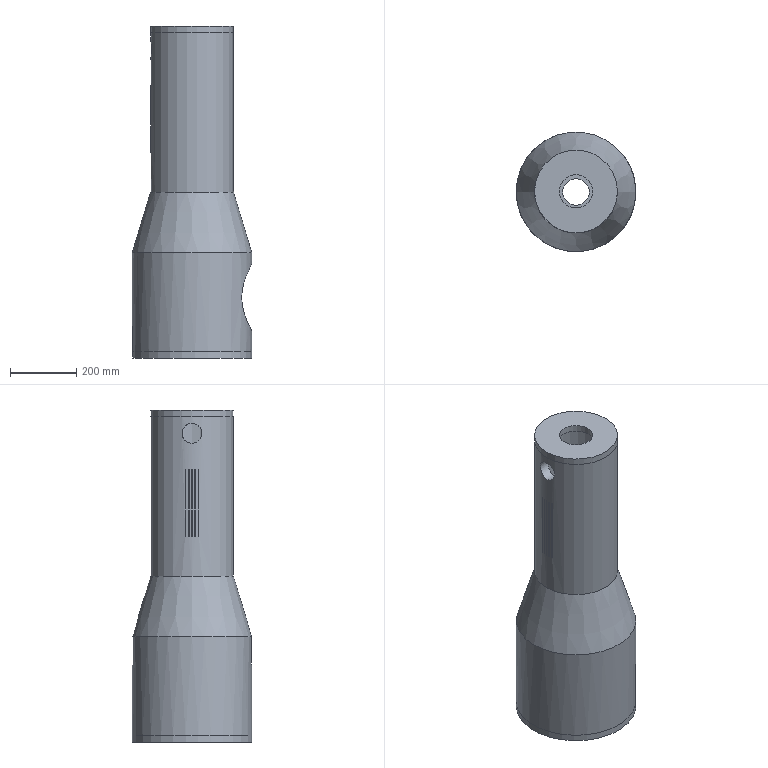Part | NX | features CYLINDER 4, DATUM_CSYS 4, EXTRUDE 3, SKETCH 3, SPLIT BODY 2, CHAMFER 1, SHELL 1 | 3 solids | 38 faces | box 360 x 360 x 1000 mm | volume 21575281 mm3 | plane 26 | cylinder 10 | cone 2 | commonest cylinder face diameters 250 x2 360 x2 60 x1 80 x1 100 x1 190 x1
STEP:
#1=CARTESIAN_POINT('',(-95.,0.,600.));
#2=VERTEX_POINT('',#1);
#3=CARTESIAN_POINT('',(-94.478,11.872,601.599));
#4=CARTESIAN_POINT('',(-95.261,-0.00341,599.201));
#5=CARTESIAN_POINT('',(-94.479,-11.859,601.595));
#6=CARTESIAN_POINT('',(-92.607,-21.764,608.254));
#7=CARTESIAN_POINT('',(-90.692,-28.404,618.148));
#8=CARTESIAN_POINT('',(-89.863,-30.794,629.974));
#9=CARTESIAN_POINT('',(-90.688,-28.419,641.834));
#10=CARTESIAN_POINT('',(-92.61,-21.752,651.761));
#11=CARTESIAN_POINT('',(-94.48,-11.846,658.408));
#12=CARTESIAN_POINT('',(-95.259,-0.01477,660.794));
#13=CARTESIAN_POINT('',(-94.483,11.831,658.417));
#14=CARTESIAN_POINT('',(-92.611,21.751,651.762));
#15=CARTESIAN_POINT('',(-90.691,28.408,641.851));
#16=CARTESIAN_POINT('',(-89.863,30.795,630.006));
#17=CARTESIAN_POINT('',(-90.69,28.413,618.159));
#18=CARTESIAN_POINT('',(-92.607,21.762,608.254));
#19=CARTESIAN_POINT('',(-94.478,11.872,601.599));
#20=CARTESIAN_POINT('',(-95.261,-0.00341,599.201));
#21=CARTESIAN_POINT('',(-94.479,-11.859,601.595));
#22=B_SPLINE_CURVE_WITH_KNOTS('',3,(#3,#4,#5,#6,#7,#8,#9,#10,#11,#12,#13,#14,#15,#16,#17,#18,#19,#20,#21),.UNSPECIFIED.,.T.,.F.,(1,1,1,1,1,1,1,1,1,1,1,1,1,1,1,1,1,1,1,1,1,1,1),(-0.0354,-0.0236,-0.0118,0.,0.0118,0.0236,0.0354,0.04719,0.05899,0.07079,0.08259,0.09439,0.1062,0.118,0.1298,0.1416,0.1534,0.1652,0.177,0.1888,0.2006,0.2124,0.2242),.UNSPECIFIED.);
#23=EDGE_CURVE('',#2,#2,#22,.T.);
#24=ORIENTED_EDGE('',*,*,#23,.T.);
#25=EDGE_LOOP('',(#24));
#26=FACE_BOUND('',#25,.T.);
#27=CARTESIAN_POINT('',(-94.573,9.,520.));
#28=VERTEX_POINT('',#27);
#29=CARTESIAN_POINT('',(-94.573,9.,320.));
#30=VERTEX_POINT('',#29);
#31=CARTESIAN_POINT('',(-94.573,9.,0.));
#32=DIRECTION('',(0.,0.,1.));
#33=VECTOR('',#32,1000.);
#34=LINE('',#31,#33);
#35=EDGE_CURVE('',#28,#30,#34,.F.);
#36=ORIENTED_EDGE('',*,*,#35,.F.);
#37=CARTESIAN_POINT('',(-94.361,11.,520.));
#38=VERTEX_POINT('',#37);
#39=CARTESIAN_POINT('',(0.,0.,520.));
#40=DIRECTION('',(0.,0.,1.));
#41=DIRECTION('',(1.,0.,0.));
#42=AXIS2_PLACEMENT_3D('',#39,#40,#41);
#43=CIRCLE('',#42,95.);
#44=EDGE_CURVE('',#38,#28,#43,.T.);
#45=ORIENTED_EDGE('',*,*,#44,.F.);
#46=CARTESIAN_POINT('',(-94.361,11.,320.));
#47=VERTEX_POINT('',#46);
#48=CARTESIAN_POINT('',(-94.361,11.,0.));
#49=DIRECTION('',(0.,0.,1.));
#50=VECTOR('',#49,1000.);
#51=LINE('',#48,#50);
#52=EDGE_CURVE('',#47,#38,#51,.T.);
#53=ORIENTED_EDGE('',*,*,#52,.F.);
#54=CARTESIAN_POINT('',(0.,0.,320.));
#55=DIRECTION('',(0.,0.,-1.));
#56=DIRECTION('',(-1.,0.,0.));
#57=AXIS2_PLACEMENT_3D('',#54,#55,#56);
#58=CIRCLE('',#57,95.);
#59=EDGE_CURVE('',#30,#47,#58,.T.);
#60=ORIENTED_EDGE('',*,*,#59,.F.);
#61=EDGE_LOOP('',(#36,#45,#53,#60));
#62=FACE_BOUND('',#61,.T.);
#63=CARTESIAN_POINT('',(-92.65,-21.,520.));
#64=VERTEX_POINT('',#63);
#65=CARTESIAN_POINT('',(-92.65,-21.,320.));
#66=VERTEX_POINT('',#65);
#67=CARTESIAN_POINT('',(-92.65,-21.,0.));
#68=DIRECTION('',(0.,0.,1.));
#69=VECTOR('',#68,1000.);
#70=LINE('',#67,#69);
#71=EDGE_CURVE('',#64,#66,#70,.F.);
#72=ORIENTED_EDGE('',*,*,#71,.F.);
#73=CARTESIAN_POINT('',(-93.081,-19.,520.));
#74=VERTEX_POINT('',#73);
#75=CARTESIAN_POINT('',(0.,0.,520.));
#76=DIRECTION('',(0.,0.,1.));
#77=DIRECTION('',(1.,0.,0.));
#78=AXIS2_PLACEMENT_3D('',#75,#76,#77);
#79=CIRCLE('',#78,95.);
#80=EDGE_CURVE('',#74,#64,#79,.T.);
#81=ORIENTED_EDGE('',*,*,#80,.F.);
#82=CARTESIAN_POINT('',(-93.081,-19.,320.));
#83=VERTEX_POINT('',#82);
#84=CARTESIAN_POINT('',(-93.081,-19.,0.));
#85=DIRECTION('',(0.,0.,1.));
#86=VECTOR('',#85,1000.);
#87=LINE('',#84,#86);
#88=EDGE_CURVE('',#83,#74,#87,.T.);
#89=ORIENTED_EDGE('',*,*,#88,.F.);
#90=CARTESIAN_POINT('',(0.,0.,320.));
#91=DIRECTION('',(0.,0.,-1.));
#92=DIRECTION('',(-1.,0.,0.));
#93=AXIS2_PLACEMENT_3D('',#90,#91,#92);
#94=CIRCLE('',#93,95.);
#95=EDGE_CURVE('',#66,#83,#94,.T.);
#96=ORIENTED_EDGE('',*,*,#95,.F.);
#97=EDGE_LOOP('',(#72,#81,#89,#96));
#98=FACE_BOUND('',#97,.T.);
#99=CARTESIAN_POINT('',(-94.995,1.,320.));
#100=VERTEX_POINT('',#99);
#101=CARTESIAN_POINT('',(-94.995,-1.,320.));
#102=VERTEX_POINT('',#101);
#103=CARTESIAN_POINT('',(0.,0.,320.));
#104=DIRECTION('',(0.,0.,-1.));
#105=DIRECTION('',(-1.,0.,0.));
#106=AXIS2_PLACEMENT_3D('',#103,#104,#105);
#107=CIRCLE('',#106,95.);
#108=EDGE_CURVE('',#100,#102,#107,.F.);
#109=ORIENTED_EDGE('',*,*,#108,.T.);
#110=CARTESIAN_POINT('',(-94.995,-1.,520.));
#111=VERTEX_POINT('',#110);
#112=CARTESIAN_POINT('',(-94.995,-1.,0.));
#113=DIRECTION('',(0.,0.,1.));
#114=VECTOR('',#113,1000.);
#115=LINE('',#112,#114);
#116=EDGE_CURVE('',#102,#111,#115,.T.);
#117=ORIENTED_EDGE('',*,*,#116,.T.);
#118=CARTESIAN_POINT('',(-94.995,1.,520.));
#119=VERTEX_POINT('',#118);
#120=CARTESIAN_POINT('',(0.,0.,520.));
#121=DIRECTION('',(0.,0.,1.));
#122=DIRECTION('',(1.,0.,0.));
#123=AXIS2_PLACEMENT_3D('',#120,#121,#122);
#124=CIRCLE('',#123,95.);
#125=EDGE_CURVE('',#111,#119,#124,.F.);
#126=ORIENTED_EDGE('',*,*,#125,.T.);
#127=CARTESIAN_POINT('',(-94.995,1.,0.));
#128=DIRECTION('',(0.,0.,1.));
#129=VECTOR('',#128,1000.);
#130=LINE('',#127,#129);
#131=EDGE_CURVE('',#119,#100,#130,.F.);
#132=ORIENTED_EDGE('',*,*,#131,.T.);
#133=EDGE_LOOP('',(#109,#117,#126,#132));
#134=FACE_BOUND('',#133,.T.);
#135=CARTESIAN_POINT('',(-95.,0.,230.398));
#136=VERTEX_POINT('',#135);
#137=CARTESIAN_POINT('',(0.,0.,230.398));
#138=DIRECTION('',(0.,0.,-1.));
#139=DIRECTION('',(-1.,0.,0.));
#140=AXIS2_PLACEMENT_3D('',#137,#138,#139);
#141=CIRCLE('',#140,95.);
#142=EDGE_CURVE('',#136,#136,#141,.F.);
#143=ORIENTED_EDGE('',*,*,#142,.F.);
#144=EDGE_LOOP('',(#143));
#145=FACE_BOUND('',#144,.T.);
#146=CARTESIAN_POINT('',(95.,0.,680.));
#147=VERTEX_POINT('',#146);
#148=CARTESIAN_POINT('',(0.,0.,680.));
#149=DIRECTION('',(0.,0.,1.));
#150=DIRECTION('',(1.,0.,0.));
#151=AXIS2_PLACEMENT_3D('',#148,#149,#150);
#152=CIRCLE('',#151,95.);
#153=EDGE_CURVE('',#147,#147,#152,.F.);
#154=ORIENTED_EDGE('',*,*,#153,.F.);
#155=EDGE_LOOP('',(#154));
#156=FACE_BOUND('',#155,.T.);
#157=CARTESIAN_POINT('',(-94.361,-11.,520.));
#158=VERTEX_POINT('',#157);
#159=CARTESIAN_POINT('',(-94.361,-11.,320.));
#160=VERTEX_POINT('',#159);
#161=CARTESIAN_POINT('',(-94.361,-11.,0.));
#162=DIRECTION('',(0.,0.,1.));
#163=VECTOR('',#162,1000.);
#164=LINE('',#161,#163);
#165=EDGE_CURVE('',#158,#160,#164,.F.);
#166=ORIENTED_EDGE('',*,*,#165,.F.);
#167=CARTESIAN_POINT('',(-94.573,-9.,520.));
#168=VERTEX_POINT('',#167);
#169=CARTESIAN_POINT('',(0.,0.,520.));
#170=DIRECTION('',(0.,0.,1.));
#171=DIRECTION('',(1.,0.,0.));
#172=AXIS2_PLACEMENT_3D('',#169,#170,#171);
#173=CIRCLE('',#172,95.);
#174=EDGE_CURVE('',#168,#158,#173,.T.);
#175=ORIENTED_EDGE('',*,*,#174,.F.);
#176=CARTESIAN_POINT('',(-94.573,-9.,320.));
#177=VERTEX_POINT('',#176);
#178=CARTESIAN_POINT('',(-94.573,-9.,0.));
#179=DIRECTION('',(0.,0.,1.));
#180=VECTOR('',#179,1000.);
#181=LINE('',#178,#180);
#182=EDGE_CURVE('',#177,#168,#181,.T.);
#183=ORIENTED_EDGE('',*,*,#182,.F.);
#184=CARTESIAN_POINT('',(0.,0.,320.));
#185=DIRECTION('',(0.,0.,-1.));
#186=DIRECTION('',(-1.,0.,0.));
#187=AXIS2_PLACEMENT_3D('',#184,#185,#186);
#188=CIRCLE('',#187,95.);
#189=EDGE_CURVE('',#160,#177,#188,.T.);
#190=ORIENTED_EDGE('',*,*,#189,.F.);
#191=EDGE_LOOP('',(#166,#175,#183,#190));
#192=FACE_BOUND('',#191,.T.);
#193=CARTESIAN_POINT('',(-93.081,19.,520.));
#194=VERTEX_POINT('',#193);
#195=CARTESIAN_POINT('',(-93.081,19.,320.));
#196=VERTEX_POINT('',#195);
#197=CARTESIAN_POINT('',(-93.081,19.,0.));
#198=DIRECTION('',(0.,0.,1.));
#199=VECTOR('',#198,1000.);
#200=LINE('',#197,#199);
#201=EDGE_CURVE('',#194,#196,#200,.F.);
#202=ORIENTED_EDGE('',*,*,#201,.F.);
#203=CARTESIAN_POINT('',(-92.65,21.,520.));
#204=VERTEX_POINT('',#203);
#205=CARTESIAN_POINT('',(0.,0.,520.));
#206=DIRECTION('',(0.,0.,1.));
#207=DIRECTION('',(1.,0.,0.));
#208=AXIS2_PLACEMENT_3D('',#205,#206,#207);
#209=CIRCLE('',#208,95.);
#210=EDGE_CURVE('',#204,#194,#209,.T.);
#211=ORIENTED_EDGE('',*,*,#210,.F.);
#212=CARTESIAN_POINT('',(-92.65,21.,320.));
#213=VERTEX_POINT('',#212);
#214=CARTESIAN_POINT('',(-92.65,21.,0.));
#215=DIRECTION('',(0.,0.,1.));
#216=VECTOR('',#215,1000.);
#217=LINE('',#214,#216);
#218=EDGE_CURVE('',#213,#204,#217,.T.);
#219=ORIENTED_EDGE('',*,*,#218,.F.);
#220=CARTESIAN_POINT('',(0.,0.,320.));
#221=DIRECTION('',(0.,0.,-1.));
#222=DIRECTION('',(-1.,0.,0.));
#223=AXIS2_PLACEMENT_3D('',#220,#221,#222);
#224=CIRCLE('',#223,95.);
#225=EDGE_CURVE('',#196,#213,#224,.T.);
#226=ORIENTED_EDGE('',*,*,#225,.F.);
#227=EDGE_LOOP('',(#202,#211,#219,#226));
#228=FACE_BOUND('',#227,.T.);
#229=CARTESIAN_POINT('',(0.,0.,0.));
#230=DIRECTION('',(0.,0.,1.));
#231=DIRECTION('',(1.,0.,0.));
#232=AXIS2_PLACEMENT_3D('',#229,#230,#231);
#233=CYLINDRICAL_SURFACE('',#232,95.);
#234=ADVANCED_FACE('',(#26,#62,#98,#134,#145,#156,#192,#228),#233,.F.);
#235=CARTESIAN_POINT('',(-125.,0.,600.));
#236=VERTEX_POINT('',#235);
#237=CARTESIAN_POINT('',(-124.604,11.861,601.594));
#238=CARTESIAN_POINT('',(-125.197,-0.008703,599.206));
#239=CARTESIAN_POINT('',(-124.606,-11.826,601.583));
#240=CARTESIAN_POINT('',(-123.189,-21.765,608.246));
#241=CARTESIAN_POINT('',(-121.754,-28.417,618.177));
#242=CARTESIAN_POINT('',(-121.144,-30.788,629.978));
#243=CARTESIAN_POINT('',(-121.75,-28.432,641.799));
#244=CARTESIAN_POINT('',(-123.19,-21.761,651.761));
#245=CARTESIAN_POINT('',(-124.607,-11.819,658.42));
#246=CARTESIAN_POINT('',(-125.196,-0.01358,660.788));
#247=CARTESIAN_POINT('',(-124.609,11.798,658.43));
#248=CARTESIAN_POINT('',(-123.193,21.743,651.776));
#249=CARTESIAN_POINT('',(-121.755,28.412,641.843));
#250=CARTESIAN_POINT('',(-121.143,30.79,630.016));
#251=CARTESIAN_POINT('',(-121.752,28.428,618.195));
#252=CARTESIAN_POINT('',(-123.188,21.77,608.255));
#253=CARTESIAN_POINT('',(-124.604,11.861,601.594));
#254=CARTESIAN_POINT('',(-125.197,-0.008703,599.206));
#255=CARTESIAN_POINT('',(-124.606,-11.826,601.583));
#256=B_SPLINE_CURVE_WITH_KNOTS('',3,(#237,#238,#239,#240,#241,#242,#243,#244,#245,#246,#247,#248,#249,#250,#251,#252,#253,#254,#255),.UNSPECIFIED.,.T.,.F.,(1,1,1,1,1,1,1,1,1,1,1,1,1,1,1,1,1,1,1,1,1,1,1),(-0.0353,-0.02353,-0.01177,0.,0.01177,0.02353,0.0353,0.04706,0.05883,0.07059,0.08236,0.09413,0.1059,0.1177,0.1294,0.1412,0.153,0.1647,0.1765,0.1883,0.2,0.2118,0.2235),.UNSPECIFIED.);
#257=EDGE_CURVE('',#236,#236,#256,.T.);
#258=ORIENTED_EDGE('',*,*,#257,.F.);
#259=EDGE_LOOP('',(#258));
#260=FACE_BOUND('',#259,.T.);
#261=CARTESIAN_POINT('',(-124.996,-1.,320.));
#262=VERTEX_POINT('',#261);
#263=CARTESIAN_POINT('',(-124.996,-1.,520.));
#264=VERTEX_POINT('',#263);
#265=CARTESIAN_POINT('',(-124.996,-1.,0.));
#266=DIRECTION('',(0.,0.,1.));
#267=VECTOR('',#266,1000.);
#268=LINE('',#265,#267);
#269=EDGE_CURVE('',#262,#264,#268,.T.);
#270=ORIENTED_EDGE('',*,*,#269,.F.);
#271=CARTESIAN_POINT('',(-124.996,1.,320.));
#272=VERTEX_POINT('',#271);
#273=CARTESIAN_POINT('',(0.,0.,320.));
#274=DIRECTION('',(0.,0.,-1.));
#275=DIRECTION('',(-1.,0.,0.));
#276=AXIS2_PLACEMENT_3D('',#273,#274,#275);
#277=CIRCLE('',#276,125.);
#278=EDGE_CURVE('',#272,#262,#277,.F.);
#279=ORIENTED_EDGE('',*,*,#278,.F.);
#280=CARTESIAN_POINT('',(-124.996,1.,520.));
#281=VERTEX_POINT('',#280);
#282=CARTESIAN_POINT('',(-124.996,1.,0.));
#283=DIRECTION('',(0.,0.,1.));
#284=VECTOR('',#283,1000.);
#285=LINE('',#282,#284);
#286=EDGE_CURVE('',#281,#272,#285,.F.);
#287=ORIENTED_EDGE('',*,*,#286,.F.);
#288=CARTESIAN_POINT('',(0.,0.,520.));
#289=DIRECTION('',(0.,0.,1.));
#290=DIRECTION('',(1.,0.,0.));
#291=AXIS2_PLACEMENT_3D('',#288,#289,#290);
#292=CIRCLE('',#291,125.);
#293=EDGE_CURVE('',#264,#281,#292,.F.);
#294=ORIENTED_EDGE('',*,*,#293,.F.);
#295=EDGE_LOOP('',(#270,#279,#287,#294));
#296=FACE_BOUND('',#295,.T.);
#297=CARTESIAN_POINT('',(-125.,0.,680.));
#298=VERTEX_POINT('',#297);
#299=CARTESIAN_POINT('',(0.,0.,680.));
#300=DIRECTION('',(0.,0.,-1.));
#301=DIRECTION('',(-1.,0.,0.));
#302=AXIS2_PLACEMENT_3D('',#299,#300,#301);
#303=CIRCLE('',#302,125.);
#304=EDGE_CURVE('',#298,#298,#303,.F.);
#305=ORIENTED_EDGE('',*,*,#304,.F.);
#306=EDGE_LOOP('',(#305));
#307=FACE_BOUND('',#306,.T.);
#308=CARTESIAN_POINT('',(125.,0.,200.));
#309=VERTEX_POINT('',#308);
#310=CARTESIAN_POINT('',(0.,0.,200.));
#311=DIRECTION('',(0.,0.,1.));
#312=DIRECTION('',(1.,0.,0.));
#313=AXIS2_PLACEMENT_3D('',#310,#311,#312);
#314=CIRCLE('',#313,125.);
#315=EDGE_CURVE('',#309,#309,#314,.T.);
#316=ORIENTED_EDGE('',*,*,#315,.T.);
#317=EDGE_LOOP('',(#316));
#318=FACE_BOUND('',#317,.T.);
#319=CARTESIAN_POINT('',(-123.548,-19.,520.));
#320=VERTEX_POINT('',#319);
#321=CARTESIAN_POINT('',(-123.223,-21.,520.));
#322=VERTEX_POINT('',#321);
#323=CARTESIAN_POINT('',(0.,0.,520.));
#324=DIRECTION('',(0.,0.,1.));
#325=DIRECTION('',(1.,0.,0.));
#326=AXIS2_PLACEMENT_3D('',#323,#324,#325);
#327=CIRCLE('',#326,125.);
#328=EDGE_CURVE('',#320,#322,#327,.T.);
#329=ORIENTED_EDGE('',*,*,#328,.T.);
#330=CARTESIAN_POINT('',(-123.223,-21.,320.));
#331=VERTEX_POINT('',#330);
#332=CARTESIAN_POINT('',(-123.223,-21.,0.));
#333=DIRECTION('',(0.,0.,1.));
#334=VECTOR('',#333,1000.);
#335=LINE('',#332,#334);
#336=EDGE_CURVE('',#322,#331,#335,.F.);
#337=ORIENTED_EDGE('',*,*,#336,.T.);
#338=CARTESIAN_POINT('',(-123.548,-19.,320.));
#339=VERTEX_POINT('',#338);
#340=CARTESIAN_POINT('',(0.,0.,320.));
#341=DIRECTION('',(0.,0.,-1.));
#342=DIRECTION('',(-1.,0.,0.));
#343=AXIS2_PLACEMENT_3D('',#340,#341,#342);
#344=CIRCLE('',#343,125.);
#345=EDGE_CURVE('',#331,#339,#344,.T.);
#346=ORIENTED_EDGE('',*,*,#345,.T.);
#347=CARTESIAN_POINT('',(-123.548,-19.,0.));
#348=DIRECTION('',(0.,0.,1.));
#349=VECTOR('',#348,1000.);
#350=LINE('',#347,#349);
#351=EDGE_CURVE('',#339,#320,#350,.T.);
#352=ORIENTED_EDGE('',*,*,#351,.T.);
#353=EDGE_LOOP('',(#329,#337,#346,#352));
#354=FACE_BOUND('',#353,.T.);
#355=CARTESIAN_POINT('',(-124.676,-9.,520.));
#356=VERTEX_POINT('',#355);
#357=CARTESIAN_POINT('',(-124.515,-11.,520.));
#358=VERTEX_POINT('',#357);
#359=CARTESIAN_POINT('',(0.,0.,520.));
#360=DIRECTION('',(0.,0.,1.));
#361=DIRECTION('',(1.,0.,0.));
#362=AXIS2_PLACEMENT_3D('',#359,#360,#361);
#363=CIRCLE('',#362,125.);
#364=EDGE_CURVE('',#356,#358,#363,.T.);
#365=ORIENTED_EDGE('',*,*,#364,.T.);
#366=CARTESIAN_POINT('',(-124.515,-11.,320.));
#367=VERTEX_POINT('',#366);
#368=CARTESIAN_POINT('',(-124.515,-11.,0.));
#369=DIRECTION('',(0.,0.,1.));
#370=VECTOR('',#369,1000.);
#371=LINE('',#368,#370);
#372=EDGE_CURVE('',#358,#367,#371,.F.);
#373=ORIENTED_EDGE('',*,*,#372,.T.);
#374=CARTESIAN_POINT('',(-124.676,-9.,320.));
#375=VERTEX_POINT('',#374);
#376=CARTESIAN_POINT('',(0.,0.,320.));
#377=DIRECTION('',(0.,0.,-1.));
#378=DIRECTION('',(-1.,0.,0.));
#379=AXIS2_PLACEMENT_3D('',#376,#377,#378);
#380=CIRCLE('',#379,125.);
#381=EDGE_CURVE('',#367,#375,#380,.T.);
#382=ORIENTED_EDGE('',*,*,#381,.T.);
#383=CARTESIAN_POINT('',(-124.676,-9.,0.));
#384=DIRECTION('',(0.,0.,1.));
#385=VECTOR('',#384,1000.);
#386=LINE('',#383,#385);
#387=EDGE_CURVE('',#375,#356,#386,.T.);
#388=ORIENTED_EDGE('',*,*,#387,.T.);
#389=EDGE_LOOP('',(#365,#373,#382,#388));
#390=FACE_BOUND('',#389,.T.);
#391=CARTESIAN_POINT('',(-124.515,11.,520.));
#392=VERTEX_POINT('',#391);
#393=CARTESIAN_POINT('',(-124.676,9.,520.));
#394=VERTEX_POINT('',#393);
#395=CARTESIAN_POINT('',(0.,0.,520.));
#396=DIRECTION('',(0.,0.,1.));
#397=DIRECTION('',(1.,0.,0.));
#398=AXIS2_PLACEMENT_3D('',#395,#396,#397);
#399=CIRCLE('',#398,125.);
#400=EDGE_CURVE('',#392,#394,#399,.T.);
#401=ORIENTED_EDGE('',*,*,#400,.T.);
#402=CARTESIAN_POINT('',(-124.676,9.,320.));
#403=VERTEX_POINT('',#402);
#404=CARTESIAN_POINT('',(-124.676,9.,0.));
#405=DIRECTION('',(0.,0.,1.));
#406=VECTOR('',#405,1000.);
#407=LINE('',#404,#406);
#408=EDGE_CURVE('',#394,#403,#407,.F.);
#409=ORIENTED_EDGE('',*,*,#408,.T.);
#410=CARTESIAN_POINT('',(-124.515,11.,320.));
#411=VERTEX_POINT('',#410);
#412=CARTESIAN_POINT('',(0.,0.,320.));
#413=DIRECTION('',(0.,0.,-1.));
#414=DIRECTION('',(-1.,0.,0.));
#415=AXIS2_PLACEMENT_3D('',#412,#413,#414);
#416=CIRCLE('',#415,125.);
#417=EDGE_CURVE('',#403,#411,#416,.T.);
#418=ORIENTED_EDGE('',*,*,#417,.T.);
#419=CARTESIAN_POINT('',(-124.515,11.,0.));
#420=DIRECTION('',(0.,0.,1.));
#421=VECTOR('',#420,1000.);
#422=LINE('',#419,#421);
#423=EDGE_CURVE('',#411,#392,#422,.T.);
#424=ORIENTED_EDGE('',*,*,#423,.T.);
#425=EDGE_LOOP('',(#401,#409,#418,#424));
#426=FACE_BOUND('',#425,.T.);
#427=CARTESIAN_POINT('',(-123.223,21.,520.));
#428=VERTEX_POINT('',#427);
#429=CARTESIAN_POINT('',(-123.548,19.,520.));
#430=VERTEX_POINT('',#429);
#431=CARTESIAN_POINT('',(0.,0.,520.));
#432=DIRECTION('',(0.,0.,1.));
#433=DIRECTION('',(1.,0.,0.));
#434=AXIS2_PLACEMENT_3D('',#431,#432,#433);
#435=CIRCLE('',#434,125.);
#436=EDGE_CURVE('',#428,#430,#435,.T.);
#437=ORIENTED_EDGE('',*,*,#436,.T.);
#438=CARTESIAN_POINT('',(-123.548,19.,320.));
#439=VERTEX_POINT('',#438);
#440=CARTESIAN_POINT('',(-123.548,19.,0.));
#441=DIRECTION('',(0.,0.,1.));
#442=VECTOR('',#441,1000.);
#443=LINE('',#440,#442);
#444=EDGE_CURVE('',#430,#439,#443,.F.);
#445=ORIENTED_EDGE('',*,*,#444,.T.);
#446=CARTESIAN_POINT('',(-123.223,21.,320.));
#447=VERTEX_POINT('',#446);
#448=CARTESIAN_POINT('',(0.,0.,320.));
#449=DIRECTION('',(0.,0.,-1.));
#450=DIRECTION('',(-1.,0.,0.));
#451=AXIS2_PLACEMENT_3D('',#448,#449,#450);
#452=CIRCLE('',#451,125.);
#453=EDGE_CURVE('',#439,#447,#452,.T.);
#454=ORIENTED_EDGE('',*,*,#453,.T.);
#455=CARTESIAN_POINT('',(-123.223,21.,0.));
#456=DIRECTION('',(0.,0.,1.));
#457=VECTOR('',#456,1000.);
#458=LINE('',#455,#457);
#459=EDGE_CURVE('',#447,#428,#458,.T.);
#460=ORIENTED_EDGE('',*,*,#459,.T.);
#461=EDGE_LOOP('',(#437,#445,#454,#460));
#462=FACE_BOUND('',#461,.T.);
#463=CARTESIAN_POINT('',(0.,0.,0.));
#464=DIRECTION('',(0.,0.,1.));
#465=DIRECTION('',(1.,0.,0.));
#466=AXIS2_PLACEMENT_3D('',#463,#464,#465);
#467=CYLINDRICAL_SURFACE('',#466,125.);
#468=ADVANCED_FACE('',(#260,#296,#307,#318,#354,#390,#426,#462),#467,.T.);
#469=CARTESIAN_POINT('',(160.,0.,-17.617));
#470=VERTEX_POINT('',#469);
#471=CARTESIAN_POINT('',(159.099,20.518,-19.051));
#472=CARTESIAN_POINT('',(160.439,-0.1034,-16.918));
#473=CARTESIAN_POINT('',(159.145,-20.104,-18.977));
#474=CARTESIAN_POINT('',(156.082,-36.139,-23.971));
#475=CARTESIAN_POINT('',(152.77,-47.832,-29.62));
#476=CARTESIAN_POINT('',(149.907,-56.148,-34.677));
#477=CARTESIAN_POINT('',(146.77,-63.875,-40.477));
#478=CARTESIAN_POINT('',(143.498,-70.901,-46.885));
#479=CARTESIAN_POINT('',(140.142,-77.308,-53.943));
#480=CARTESIAN_POINT('',(135.688,-84.973,-64.228));
#481=CARTESIAN_POINT('',(130.613,-92.568,-78.149));
#482=CARTESIAN_POINT('',(126.812,-97.586,-94.068));
#483=CARTESIAN_POINT('',(125.2,-99.627,-107.205));
#484=CARTESIAN_POINT('',(124.615,-100.352,-120.826));
#485=CARTESIAN_POINT('',(125.697,-99.022,-134.142));
#486=CARTESIAN_POINT('',(128.229,-95.717,-147.132));
#487=CARTESIAN_POINT('',(131.48,-91.262,-159.395));
#488=CARTESIAN_POINT('',(136.655,-83.532,-173.697));
#489=CARTESIAN_POINT('',(142.28,-73.495,-185.953));
#490=CARTESIAN_POINT('',(146.709,-64.017,-194.64));
#491=CARTESIAN_POINT('',(149.814,-56.386,-200.387));
#492=CARTESIAN_POINT('',(152.658,-48.191,-205.419));
#493=CARTESIAN_POINT('',(155.183,-39.341,-209.731));
#494=CARTESIAN_POINT('',(157.258,-30.015,-213.178));
#495=CARTESIAN_POINT('',(158.789,-20.444,-215.671));
#496=CARTESIAN_POINT('',(159.758,-10.572,-217.23));
#497=CARTESIAN_POINT('',(160.223,3.07,-217.972));
#498=CARTESIAN_POINT('',(159.402,16.372,-216.668));
#499=CARTESIAN_POINT('',(157.365,29.465,-213.353));
#500=CARTESIAN_POINT('',(155.328,38.755,-209.975));
#501=CARTESIAN_POINT('',(152.843,47.606,-205.742));
#502=CARTESIAN_POINT('',(149.005,58.786,-198.965));
#503=CARTESIAN_POINT('',(144.7,68.597,-190.869));
#504=CARTESIAN_POINT('',(140.176,77.247,-181.364));
#505=CARTESIAN_POINT('',(136.866,82.95,-173.736));
#506=CARTESIAN_POINT('',(133.716,87.921,-165.582));
#507=CARTESIAN_POINT('',(130.816,92.166,-156.831));
#508=CARTESIAN_POINT('',(128.328,95.585,-147.546));
#509=CARTESIAN_POINT('',(125.788,98.908,-134.799));
#510=CARTESIAN_POINT('',(124.63,100.334,-121.166));
#511=CARTESIAN_POINT('',(125.151,99.689,-107.816));
#512=CARTESIAN_POINT('',(126.74,97.678,-94.412));
#513=CARTESIAN_POINT('',(129.709,93.774,-81.822));
#514=CARTESIAN_POINT('',(133.58,88.129,-70.026));
#515=CARTESIAN_POINT('',(136.738,83.16,-61.808));
#516=CARTESIAN_POINT('',(140.058,77.46,-54.127));
#517=CARTESIAN_POINT('',(144.585,68.836,-44.591));
#518=CARTESIAN_POINT('',(149.963,56.656,-34.456));
#519=CARTESIAN_POINT('',(155.476,39.283,-24.958));
#520=CARTESIAN_POINT('',(159.099,20.518,-19.051));
#521=CARTESIAN_POINT('',(160.439,-0.1034,-16.918));
#522=CARTESIAN_POINT('',(159.145,-20.104,-18.977));
#523=B_SPLINE_CURVE_WITH_KNOTS('',3,(#471,#472,#473,#474,#475,#476,#477,#478,#479,#480,#481,#482,#483,#484,#485,#486,#487,#488,#489,#490,#491,#492,#493,#494,#495,#496,#497,#498,#499,#500,#501,#502,#503,#504,#505,#506,#507,#508,#509,#510,#511,#512,#513,#514,#515,#516,#517,#518,#519,#520,#521,#522),.UNSPECIFIED.,.T.,.F.,(1,1,1,1,1,1,1,1,1,1,1,1,1,1,1,1,1,1,1,1,1,1,1,1,1,1,1,1,1,1,1,1,1,1,1,1,1,1,1,1,1,1,1,1,1,1,1,1,1,1,1,1,1,1,1,1),(-0.06025,-0.04016,-0.02008,0.,0.02008,0.04016,0.05021,0.06025,0.07029,0.08033,0.09037,0.1004,0.1205,0.1406,0.1506,0.1607,0.1807,0.1908,0.2008,0.2209,0.241,0.251,0.2611,0.2711,0.2812,0.2912,0.3012,0.3113,0.3213,0.3414,0.3514,0.3615,0.3715,0.3816,0.4016,0.4117,0.4217,0.4318,0.4418,0.4518,0.4619,0.482,0.492,0.5021,0.5221,0.5322,0.5422,0.5523,0.5623,0.5824,0.6025,0.6225,0.6426,0.6627,0.6828,0.6928),.UNSPECIFIED.);
#524=EDGE_CURVE('',#470,#470,#523,.T.);
#525=ORIENTED_EDGE('',*,*,#524,.T.);
#526=EDGE_LOOP('',(#525));
#527=FACE_BOUND('',#526,.T.);
#528=CARTESIAN_POINT('',(-160.,0.,13.731));
#529=VERTEX_POINT('',#528);
#530=CARTESIAN_POINT('',(0.,0.,13.731));
#531=DIRECTION('',(0.,0.,-1.));
#532=DIRECTION('',(-1.,0.,0.));
#533=AXIS2_PLACEMENT_3D('',#530,#531,#532);
#534=CIRCLE('',#533,160.);
#535=EDGE_CURVE('',#529,#529,#534,.T.);
#536=ORIENTED_EDGE('',*,*,#535,.F.);
#537=EDGE_LOOP('',(#536));
#538=FACE_BOUND('',#537,.T.);
#539=CARTESIAN_POINT('',(-160.,0.,-280.));
#540=VERTEX_POINT('',#539);
#541=CARTESIAN_POINT('',(0.,0.,-280.));
#542=DIRECTION('',(0.,0.,-1.));
#543=DIRECTION('',(-1.,0.,0.));
#544=AXIS2_PLACEMENT_3D('',#541,#542,#543);
#545=CIRCLE('',#544,160.);
#546=EDGE_CURVE('',#540,#540,#545,.F.);
#547=ORIENTED_EDGE('',*,*,#546,.F.);
#548=EDGE_LOOP('',(#547));
#549=FACE_BOUND('',#548,.T.);
#550=CARTESIAN_POINT('',(0.,0.,0.));
#551=DIRECTION('',(0.,0.,-1.));
#552=DIRECTION('',(1.,0.,0.));
#553=AXIS2_PLACEMENT_3D('',#550,#551,#552);
#554=CYLINDRICAL_SURFACE('',#553,160.);
#555=ADVANCED_FACE('',(#527,#538,#549),#554,.F.);
#556=ORIENTED_EDGE('',*,*,#142,.T.);
#557=EDGE_LOOP('',(#556));
#558=FACE_BOUND('',#557,.T.);
#559=ORIENTED_EDGE('',*,*,#535,.T.);
#560=EDGE_LOOP('',(#559));
#561=FACE_BOUND('',#560,.T.);
#562=CARTESIAN_POINT('',(0.,0.,-5.747));
#563=DIRECTION('',(0.,0.,-1.));
#564=DIRECTION('',(-1.,0.,0.));
#565=AXIS2_PLACEMENT_3D('',#562,#563,#564);
#566=CONICAL_SURFACE('',#565,165.843,0.2915);
#567=ADVANCED_FACE('',(#558,#561),#566,.F.);
#568=CARTESIAN_POINT('',(180.,0.,-17.617));
#569=VERTEX_POINT('',#568);
#570=CARTESIAN_POINT('',(179.809,10.097,-17.96));
#571=CARTESIAN_POINT('',(180.095,-0.006015,-17.445));
#572=CARTESIAN_POINT('',(179.809,-10.073,-17.959));
#573=CARTESIAN_POINT('',(178.716,-23.155,-19.938));
#574=CARTESIAN_POINT('',(176.022,-39.153,-24.896));
#575=CARTESIAN_POINT('',(172.059,-53.393,-32.632));
#576=CARTESIAN_POINT('',(168.379,-63.795,-40.406));
#577=CARTESIAN_POINT('',(165.516,-70.869,-46.851));
#578=CARTESIAN_POINT('',(162.6,-77.308,-53.941));
#579=CARTESIAN_POINT('',(158.737,-85.044,-64.323));
#580=CARTESIAN_POINT('',(155.267,-91.139,-75.581));
#581=CARTESIAN_POINT('',(152.497,-95.649,-87.879));
#582=CARTESIAN_POINT('',(150.899,-98.139,-97.574));
#583=CARTESIAN_POINT('',(149.907,-99.641,-107.381));
#584=CARTESIAN_POINT('',(149.551,-100.171,-117.455));
#585=CARTESIAN_POINT('',(149.886,-99.673,-127.546));
#586=CARTESIAN_POINT('',(151.183,-97.71,-140.64));
#587=CARTESIAN_POINT('',(153.697,-93.771,-153.413));
#588=CARTESIAN_POINT('',(156.941,-88.198,-165.079));
#589=CARTESIAN_POINT('',(160.59,-81.476,-176.222));
#590=CARTESIAN_POINT('',(165.473,-71.362,-188.549));
#591=CARTESIAN_POINT('',(171.233,-56.34,-200.986));
#592=CARTESIAN_POINT('',(175.173,-42.221,-208.683));
#593=CARTESIAN_POINT('',(177.615,-29.737,-213.268));
#594=CARTESIAN_POINT('',(178.962,-20.108,-215.74));
#595=CARTESIAN_POINT('',(179.796,-10.31,-217.25));
#596=CARTESIAN_POINT('',(180.095,-0.2804,-217.787));
#597=CARTESIAN_POINT('',(179.823,9.851,-217.299));
#598=CARTESIAN_POINT('',(179.01,19.687,-215.827));
#599=CARTESIAN_POINT('',(177.677,29.363,-213.383));
#600=CARTESIAN_POINT('',(175.262,41.855,-208.853));
#601=CARTESIAN_POINT('',(172.094,53.283,-202.673));
#602=CARTESIAN_POINT('',(168.413,63.705,-194.902));
#603=CARTESIAN_POINT('',(165.548,70.795,-188.457));
#604=CARTESIAN_POINT('',(162.627,77.253,-181.361));
#605=CARTESIAN_POINT('',(158.757,85.006,-170.968));
#606=CARTESIAN_POINT('',(154.41,92.645,-156.918));
#607=CARTESIAN_POINT('',(151.233,97.634,-140.967));
#608=CARTESIAN_POINT('',(149.907,99.641,-127.862));
#609=CARTESIAN_POINT('',(149.551,100.172,-117.761));
#610=CARTESIAN_POINT('',(149.887,99.671,-107.671));
#611=CARTESIAN_POINT('',(151.188,97.702,-94.556));
#612=CARTESIAN_POINT('',(153.708,93.752,-81.77));
#613=CARTESIAN_POINT('',(156.961,88.164,-70.091));
#614=CARTESIAN_POINT('',(160.619,81.422,-58.933));
#615=CARTESIAN_POINT('',(165.507,71.286,-46.606));
#616=CARTESIAN_POINT('',(171.271,56.225,-34.168));
#617=CARTESIAN_POINT('',(175.209,42.075,-26.482));
#618=CARTESIAN_POINT('',(177.646,29.552,-21.908));
#619=CARTESIAN_POINT('',(178.984,19.914,-19.453));
#620=CARTESIAN_POINT('',(179.809,10.097,-17.96));
#621=CARTESIAN_POINT('',(180.095,-0.006015,-17.445));
#622=CARTESIAN_POINT('',(179.809,-10.073,-17.959));
#623=B_SPLINE_CURVE_WITH_KNOTS('',3,(#570,#571,#572,#573,#574,#575,#576,#577,#578,#579,#580,#581,#582,#583,#584,#585,#586,#587,#588,#589,#590,#591,#592,#593,#594,#595,#596,#597,#598,#599,#600,#601,#602,#603,#604,#605,#606,#607,#608,#609,#610,#611,#612,#613,#614,#615,#616,#617,#618,#619,#620,#621,#622),.UNSPECIFIED.,.T.,.F.,(1,1,1,1,1,1,1,1,1,1,1,1,1,1,1,1,1,1,1,1,1,1,1,1,1,1,1,1,1,1,1,1,1,1,1,1,1,1,1,1,1,1,1,1,1,1,1,1,1,1,1,1,1,1,1,1,1),(-0.02993,-0.01995,-0.009976,0.,0.009976,0.01995,0.0399,0.05986,0.06983,0.07981,0.08978,0.09976,0.1197,0.1297,0.1397,0.1496,0.1596,0.1696,0.1796,0.1995,0.2095,0.2195,0.2394,0.2594,0.2793,0.2893,0.2993,0.3093,0.3192,0.3292,0.3392,0.3492,0.3591,0.3791,0.3891,0.399,0.409,0.419,0.4389,0.4589,0.4689,0.4788,0.4888,0.4988,0.5187,0.5287,0.5387,0.5587,0.5786,0.5986,0.6085,0.6185,0.6285,0.6385,0.6484,0.6584,0.6784),.UNSPECIFIED.);
#624=EDGE_CURVE('',#569,#569,#623,.T.);
#625=ORIENTED_EDGE('',*,*,#624,.F.);
#626=EDGE_LOOP('',(#625));
#627=FACE_BOUND('',#626,.T.);
#628=CARTESIAN_POINT('',(180.,0.,-280.));
#629=VERTEX_POINT('',#628);
#630=CARTESIAN_POINT('',(0.,0.,-280.));
#631=DIRECTION('',(0.,0.,1.));
#632=DIRECTION('',(1.,0.,0.));
#633=AXIS2_PLACEMENT_3D('',#630,#631,#632);
#634=CIRCLE('',#633,180.);
#635=EDGE_CURVE('',#629,#629,#634,.F.);
#636=ORIENTED_EDGE('',*,*,#635,.F.);
#637=EDGE_LOOP('',(#636));
#638=FACE_BOUND('',#637,.T.);
#639=CARTESIAN_POINT('',(-180.,0.,16.667));
#640=VERTEX_POINT('',#639);
#641=CARTESIAN_POINT('',(0.,0.,16.667));
#642=DIRECTION('',(0.,0.,-1.));
#643=DIRECTION('',(-1.,0.,0.));
#644=AXIS2_PLACEMENT_3D('',#641,#642,#643);
#645=CIRCLE('',#644,180.);
#646=EDGE_CURVE('',#640,#640,#645,.T.);
#647=ORIENTED_EDGE('',*,*,#646,.T.);
#648=EDGE_LOOP('',(#647));
#649=FACE_BOUND('',#648,.T.);
#650=CARTESIAN_POINT('',(0.,0.,0.));
#651=DIRECTION('',(0.,0.,-1.));
#652=DIRECTION('',(1.,0.,0.));
#653=AXIS2_PLACEMENT_3D('',#650,#651,#652);
#654=CYLINDRICAL_SURFACE('',#653,180.);
#655=ADVANCED_FACE('',(#627,#638,#649),#654,.T.);
#656=ORIENTED_EDGE('',*,*,#315,.F.);
#657=EDGE_LOOP('',(#656));
#658=FACE_BOUND('',#657,.T.);
#659=ORIENTED_EDGE('',*,*,#646,.F.);
#660=EDGE_LOOP('',(#659));
#661=FACE_BOUND('',#660,.T.);
#662=CARTESIAN_POINT('',(0.,0.,0.));
#663=DIRECTION('',(0.,0.,-1.));
#664=DIRECTION('',(-1.,0.,0.));
#665=AXIS2_PLACEMENT_3D('',#662,#663,#664);
#666=CONICAL_SURFACE('',#665,185.,0.2915);
#667=ADVANCED_FACE('',(#658,#661),#666,.T.);
#668=ORIENTED_EDGE('',*,*,#546,.T.);
#669=EDGE_LOOP('',(#668));
#670=FACE_BOUND('',#669,.T.);
#671=ORIENTED_EDGE('',*,*,#635,.T.);
#672=EDGE_LOOP('',(#671));
#673=FACE_BOUND('',#672,.T.);
#674=CARTESIAN_POINT('',(0.,0.,-280.));
#675=DIRECTION('',(0.,0.,1.));
#676=DIRECTION('',(1.,0.,0.));
#677=AXIS2_PLACEMENT_3D('',#674,#675,#676);
#678=PLANE('',#677);
#679=ADVANCED_FACE('',(#670,#673),#678,.F.);
#680=ORIENTED_EDGE('',*,*,#153,.T.);
#681=EDGE_LOOP('',(#680));
#682=FACE_BOUND('',#681,.T.);
#683=ORIENTED_EDGE('',*,*,#304,.T.);
#684=EDGE_LOOP('',(#683));
#685=FACE_BOUND('',#684,.T.);
#686=CARTESIAN_POINT('',(0.,0.,680.));
#687=DIRECTION('',(0.,0.,-1.));
#688=DIRECTION('',(-1.,0.,0.));
#689=AXIS2_PLACEMENT_3D('',#686,#687,#688);
#690=PLANE('',#689);
#691=ADVANCED_FACE('',(#682,#685),#690,.F.);
#692=ORIENTED_EDGE('',*,*,#624,.T.);
#693=EDGE_LOOP('',(#692));
#694=FACE_BOUND('',#693,.T.);
#695=ORIENTED_EDGE('',*,*,#524,.F.);
#696=EDGE_LOOP('',(#695));
#697=FACE_BOUND('',#696,.T.);
#698=CARTESIAN_POINT('',(230.,0.,-117.617));
#699=DIRECTION('',(-1.,0.,0.));
#700=DIRECTION('',(0.,0.,1.));
#701=AXIS2_PLACEMENT_3D('',#698,#699,#700);
#702=CYLINDRICAL_SURFACE('',#701,100.);
#703=ADVANCED_FACE('',(#694,#697),#702,.F.);
#704=CARTESIAN_POINT('',(0.,-1.,320.));
#705=DIRECTION('',(1.,0.,0.));
#706=VECTOR('',#705,1000.);
#707=LINE('',#704,#706);
#708=EDGE_CURVE('',#102,#262,#707,.F.);
#709=ORIENTED_EDGE('',*,*,#708,.T.);
#710=ORIENTED_EDGE('',*,*,#269,.T.);
#711=CARTESIAN_POINT('',(0.,-1.,520.));
#712=DIRECTION('',(1.,0.,0.));
#713=VECTOR('',#712,1000.);
#714=LINE('',#711,#713);
#715=EDGE_CURVE('',#111,#264,#714,.F.);
#716=ORIENTED_EDGE('',*,*,#715,.F.);
#717=ORIENTED_EDGE('',*,*,#116,.F.);
#718=EDGE_LOOP('',(#709,#710,#716,#717));
#719=FACE_BOUND('',#718,.T.);
#720=CARTESIAN_POINT('',(0.,-1.,520.));
#721=DIRECTION('',(0.,-1.,0.));
#722=DIRECTION('',(0.,0.,-1.));
#723=AXIS2_PLACEMENT_3D('',#720,#721,#722);
#724=PLANE('',#723);
#725=ADVANCED_FACE('',(#719),#724,.F.);
#726=CARTESIAN_POINT('',(0.,1.,320.));
#727=DIRECTION('',(1.,0.,0.));
#728=VECTOR('',#727,1000.);
#729=LINE('',#726,#728);
#730=EDGE_CURVE('',#100,#272,#729,.F.);
#731=ORIENTED_EDGE('',*,*,#730,.T.);
#732=ORIENTED_EDGE('',*,*,#278,.T.);
#733=ORIENTED_EDGE('',*,*,#708,.F.);
#734=ORIENTED_EDGE('',*,*,#108,.F.);
#735=EDGE_LOOP('',(#731,#732,#733,#734));
#736=FACE_BOUND('',#735,.T.);
#737=CARTESIAN_POINT('',(0.,-1.,320.));
#738=DIRECTION('',(0.,0.,-1.));
#739=DIRECTION('',(-1.,0.,0.));
#740=AXIS2_PLACEMENT_3D('',#737,#738,#739);
#741=PLANE('',#740);
#742=ADVANCED_FACE('',(#736),#741,.F.);
#743=CARTESIAN_POINT('',(0.,1.,520.));
#744=DIRECTION('',(1.,0.,0.));
#745=VECTOR('',#744,1000.);
#746=LINE('',#743,#745);
#747=EDGE_CURVE('',#119,#281,#746,.F.);
#748=ORIENTED_EDGE('',*,*,#747,.T.);
#749=ORIENTED_EDGE('',*,*,#286,.T.);
#750=ORIENTED_EDGE('',*,*,#730,.F.);
#751=ORIENTED_EDGE('',*,*,#131,.F.);
#752=EDGE_LOOP('',(#748,#749,#750,#751));
#753=FACE_BOUND('',#752,.T.);
#754=CARTESIAN_POINT('',(0.,1.,520.));
#755=DIRECTION('',(0.,1.,0.));
#756=DIRECTION('',(0.,0.,1.));
#757=AXIS2_PLACEMENT_3D('',#754,#755,#756);
#758=PLANE('',#757);
#759=ADVANCED_FACE('',(#753),#758,.F.);
#760=ORIENTED_EDGE('',*,*,#715,.T.);
#761=ORIENTED_EDGE('',*,*,#293,.T.);
#762=ORIENTED_EDGE('',*,*,#747,.F.);
#763=ORIENTED_EDGE('',*,*,#125,.F.);
#764=EDGE_LOOP('',(#760,#761,#762,#763));
#765=FACE_BOUND('',#764,.T.);
#766=CARTESIAN_POINT('',(0.,-1.,520.));
#767=DIRECTION('',(0.,0.,1.));
#768=DIRECTION('',(1.,0.,0.));
#769=AXIS2_PLACEMENT_3D('',#766,#767,#768);
#770=PLANE('',#769);
#771=ADVANCED_FACE('',(#765),#770,.F.);
#772=ORIENTED_EDGE('',*,*,#71,.T.);
#773=CARTESIAN_POINT('',(0.,-21.,320.));
#774=DIRECTION('',(1.,0.,0.));
#775=VECTOR('',#774,1000.);
#776=LINE('',#773,#775);
#777=EDGE_CURVE('',#66,#331,#776,.F.);
#778=ORIENTED_EDGE('',*,*,#777,.T.);
#779=ORIENTED_EDGE('',*,*,#336,.F.);
#780=CARTESIAN_POINT('',(0.,-21.,520.));
#781=DIRECTION('',(1.,0.,0.));
#782=VECTOR('',#781,1000.);
#783=LINE('',#780,#782);
#784=EDGE_CURVE('',#64,#322,#783,.F.);
#785=ORIENTED_EDGE('',*,*,#784,.F.);
#786=EDGE_LOOP('',(#772,#778,#779,#785));
#787=FACE_BOUND('',#786,.T.);
#788=CARTESIAN_POINT('',(0.,-21.,320.));
#789=DIRECTION('',(0.,-1.,0.));
#790=DIRECTION('',(0.,0.,-1.));
#791=AXIS2_PLACEMENT_3D('',#788,#789,#790);
#792=PLANE('',#791);
#793=ADVANCED_FACE('',(#787),#792,.F.);
#794=ORIENTED_EDGE('',*,*,#80,.T.);
#795=ORIENTED_EDGE('',*,*,#784,.T.);
#796=ORIENTED_EDGE('',*,*,#328,.F.);
#797=CARTESIAN_POINT('',(0.,-19.,520.));
#798=DIRECTION('',(1.,0.,0.));
#799=VECTOR('',#798,1000.);
#800=LINE('',#797,#799);
#801=EDGE_CURVE('',#74,#320,#800,.F.);
#802=ORIENTED_EDGE('',*,*,#801,.F.);
#803=EDGE_LOOP('',(#794,#795,#796,#802));
#804=FACE_BOUND('',#803,.T.);
#805=CARTESIAN_POINT('',(0.,-21.,520.));
#806=DIRECTION('',(0.,0.,1.));
#807=DIRECTION('',(1.,0.,0.));
#808=AXIS2_PLACEMENT_3D('',#805,#806,#807);
#809=PLANE('',#808);
#810=ADVANCED_FACE('',(#804),#809,.F.);
#811=ORIENTED_EDGE('',*,*,#88,.T.);
#812=ORIENTED_EDGE('',*,*,#801,.T.);
#813=ORIENTED_EDGE('',*,*,#351,.F.);
#814=CARTESIAN_POINT('',(0.,-19.,320.));
#815=DIRECTION('',(1.,0.,0.));
#816=VECTOR('',#815,1000.);
#817=LINE('',#814,#816);
#818=EDGE_CURVE('',#83,#339,#817,.F.);
#819=ORIENTED_EDGE('',*,*,#818,.F.);
#820=EDGE_LOOP('',(#811,#812,#813,#819));
#821=FACE_BOUND('',#820,.T.);
#822=CARTESIAN_POINT('',(0.,-19.,320.));
#823=DIRECTION('',(0.,1.,0.));
#824=DIRECTION('',(0.,0.,1.));
#825=AXIS2_PLACEMENT_3D('',#822,#823,#824);
#826=PLANE('',#825);
#827=ADVANCED_FACE('',(#821),#826,.F.);
#828=ORIENTED_EDGE('',*,*,#95,.T.);
#829=ORIENTED_EDGE('',*,*,#818,.T.);
#830=ORIENTED_EDGE('',*,*,#345,.F.);
#831=ORIENTED_EDGE('',*,*,#777,.F.);
#832=EDGE_LOOP('',(#828,#829,#830,#831));
#833=FACE_BOUND('',#832,.T.);
#834=CARTESIAN_POINT('',(0.,-21.,320.));
#835=DIRECTION('',(0.,0.,-1.));
#836=DIRECTION('',(-1.,0.,0.));
#837=AXIS2_PLACEMENT_3D('',#834,#835,#836);
#838=PLANE('',#837);
#839=ADVANCED_FACE('',(#833),#838,.F.);
#840=ORIENTED_EDGE('',*,*,#165,.T.);
#841=CARTESIAN_POINT('',(0.,-11.,320.));
#842=DIRECTION('',(1.,0.,0.));
#843=VECTOR('',#842,1000.);
#844=LINE('',#841,#843);
#845=EDGE_CURVE('',#160,#367,#844,.F.);
#846=ORIENTED_EDGE('',*,*,#845,.T.);
#847=ORIENTED_EDGE('',*,*,#372,.F.);
#848=CARTESIAN_POINT('',(0.,-11.,520.));
#849=DIRECTION('',(1.,0.,0.));
#850=VECTOR('',#849,1000.);
#851=LINE('',#848,#850);
#852=EDGE_CURVE('',#158,#358,#851,.F.);
#853=ORIENTED_EDGE('',*,*,#852,.F.);
#854=EDGE_LOOP('',(#840,#846,#847,#853));
#855=FACE_BOUND('',#854,.T.);
#856=CARTESIAN_POINT('',(0.,-11.,320.));
#857=DIRECTION('',(0.,-1.,0.));
#858=DIRECTION('',(0.,0.,-1.));
#859=AXIS2_PLACEMENT_3D('',#856,#857,#858);
#860=PLANE('',#859);
#861=ADVANCED_FACE('',(#855),#860,.F.);
#862=ORIENTED_EDGE('',*,*,#174,.T.);
#863=ORIENTED_EDGE('',*,*,#852,.T.);
#864=ORIENTED_EDGE('',*,*,#364,.F.);
#865=CARTESIAN_POINT('',(0.,-9.,520.));
#866=DIRECTION('',(1.,0.,0.));
#867=VECTOR('',#866,1000.);
#868=LINE('',#865,#867);
#869=EDGE_CURVE('',#168,#356,#868,.F.);
#870=ORIENTED_EDGE('',*,*,#869,.F.);
#871=EDGE_LOOP('',(#862,#863,#864,#870));
#872=FACE_BOUND('',#871,.T.);
#873=CARTESIAN_POINT('',(0.,-11.,520.));
#874=DIRECTION('',(0.,0.,1.));
#875=DIRECTION('',(1.,0.,0.));
#876=AXIS2_PLACEMENT_3D('',#873,#874,#875);
#877=PLANE('',#876);
#878=ADVANCED_FACE('',(#872),#877,.F.);
#879=ORIENTED_EDGE('',*,*,#182,.T.);
#880=ORIENTED_EDGE('',*,*,#869,.T.);
#881=ORIENTED_EDGE('',*,*,#387,.F.);
#882=CARTESIAN_POINT('',(0.,-9.,320.));
#883=DIRECTION('',(1.,0.,0.));
#884=VECTOR('',#883,1000.);
#885=LINE('',#882,#884);
#886=EDGE_CURVE('',#177,#375,#885,.F.);
#887=ORIENTED_EDGE('',*,*,#886,.F.);
#888=EDGE_LOOP('',(#879,#880,#881,#887));
#889=FACE_BOUND('',#888,.T.);
#890=CARTESIAN_POINT('',(0.,-9.,320.));
#891=DIRECTION('',(0.,1.,0.));
#892=DIRECTION('',(0.,0.,1.));
#893=AXIS2_PLACEMENT_3D('',#890,#891,#892);
#894=PLANE('',#893);
#895=ADVANCED_FACE('',(#889),#894,.F.);
#896=ORIENTED_EDGE('',*,*,#189,.T.);
#897=ORIENTED_EDGE('',*,*,#886,.T.);
#898=ORIENTED_EDGE('',*,*,#381,.F.);
#899=ORIENTED_EDGE('',*,*,#845,.F.);
#900=EDGE_LOOP('',(#896,#897,#898,#899));
#901=FACE_BOUND('',#900,.T.);
#902=CARTESIAN_POINT('',(0.,-11.,320.));
#903=DIRECTION('',(0.,0.,-1.));
#904=DIRECTION('',(-1.,0.,0.));
#905=AXIS2_PLACEMENT_3D('',#902,#903,#904);
#906=PLANE('',#905);
#907=ADVANCED_FACE('',(#901),#906,.F.);
#908=ORIENTED_EDGE('',*,*,#35,.T.);
#909=CARTESIAN_POINT('',(0.,9.,320.));
#910=DIRECTION('',(1.,0.,0.));
#911=VECTOR('',#910,1000.);
#912=LINE('',#909,#911);
#913=EDGE_CURVE('',#30,#403,#912,.F.);
#914=ORIENTED_EDGE('',*,*,#913,.T.);
#915=ORIENTED_EDGE('',*,*,#408,.F.);
#916=CARTESIAN_POINT('',(0.,9.,520.));
#917=DIRECTION('',(1.,0.,0.));
#918=VECTOR('',#917,1000.);
#919=LINE('',#916,#918);
#920=EDGE_CURVE('',#28,#394,#919,.F.);
#921=ORIENTED_EDGE('',*,*,#920,.F.);
#922=EDGE_LOOP('',(#908,#914,#915,#921));
#923=FACE_BOUND('',#922,.T.);
#924=CARTESIAN_POINT('',(0.,9.,320.));
#925=DIRECTION('',(0.,-1.,0.));
#926=DIRECTION('',(0.,0.,-1.));
#927=AXIS2_PLACEMENT_3D('',#924,#925,#926);
#928=PLANE('',#927);
#929=ADVANCED_FACE('',(#923),#928,.F.);
#930=ORIENTED_EDGE('',*,*,#44,.T.);
#931=ORIENTED_EDGE('',*,*,#920,.T.);
#932=ORIENTED_EDGE('',*,*,#400,.F.);
#933=CARTESIAN_POINT('',(0.,11.,520.));
#934=DIRECTION('',(1.,0.,0.));
#935=VECTOR('',#934,1000.);
#936=LINE('',#933,#935);
#937=EDGE_CURVE('',#38,#392,#936,.F.);
#938=ORIENTED_EDGE('',*,*,#937,.F.);
#939=EDGE_LOOP('',(#930,#931,#932,#938));
#940=FACE_BOUND('',#939,.T.);
#941=CARTESIAN_POINT('',(0.,9.,520.));
#942=DIRECTION('',(0.,0.,1.));
#943=DIRECTION('',(1.,0.,0.));
#944=AXIS2_PLACEMENT_3D('',#941,#942,#943);
#945=PLANE('',#944);
#946=ADVANCED_FACE('',(#940),#945,.F.);
#947=ORIENTED_EDGE('',*,*,#52,.T.);
#948=ORIENTED_EDGE('',*,*,#937,.T.);
#949=ORIENTED_EDGE('',*,*,#423,.F.);
#950=CARTESIAN_POINT('',(0.,11.,320.));
#951=DIRECTION('',(1.,0.,0.));
#952=VECTOR('',#951,1000.);
#953=LINE('',#950,#952);
#954=EDGE_CURVE('',#47,#411,#953,.F.);
#955=ORIENTED_EDGE('',*,*,#954,.F.);
#956=EDGE_LOOP('',(#947,#948,#949,#955));
#957=FACE_BOUND('',#956,.T.);
#958=CARTESIAN_POINT('',(0.,11.,320.));
#959=DIRECTION('',(0.,1.,0.));
#960=DIRECTION('',(0.,0.,1.));
#961=AXIS2_PLACEMENT_3D('',#958,#959,#960);
#962=PLANE('',#961);
#963=ADVANCED_FACE('',(#957),#962,.F.);
#964=ORIENTED_EDGE('',*,*,#59,.T.);
#965=ORIENTED_EDGE('',*,*,#954,.T.);
#966=ORIENTED_EDGE('',*,*,#417,.F.);
#967=ORIENTED_EDGE('',*,*,#913,.F.);
#968=EDGE_LOOP('',(#964,#965,#966,#967));
#969=FACE_BOUND('',#968,.T.);
#970=CARTESIAN_POINT('',(0.,9.,320.));
#971=DIRECTION('',(0.,0.,-1.));
#972=DIRECTION('',(-1.,0.,0.));
#973=AXIS2_PLACEMENT_3D('',#970,#971,#972);
#974=PLANE('',#973);
#975=ADVANCED_FACE('',(#969),#974,.F.);
#976=ORIENTED_EDGE('',*,*,#201,.T.);
#977=CARTESIAN_POINT('',(0.,19.,320.));
#978=DIRECTION('',(1.,0.,0.));
#979=VECTOR('',#978,1000.);
#980=LINE('',#977,#979);
#981=EDGE_CURVE('',#196,#439,#980,.F.);
#982=ORIENTED_EDGE('',*,*,#981,.T.);
#983=ORIENTED_EDGE('',*,*,#444,.F.);
#984=CARTESIAN_POINT('',(0.,19.,520.));
#985=DIRECTION('',(1.,0.,0.));
#986=VECTOR('',#985,1000.);
#987=LINE('',#984,#986);
#988=EDGE_CURVE('',#194,#430,#987,.F.);
#989=ORIENTED_EDGE('',*,*,#988,.F.);
#990=EDGE_LOOP('',(#976,#982,#983,#989));
#991=FACE_BOUND('',#990,.T.);
#992=CARTESIAN_POINT('',(0.,19.,320.));
#993=DIRECTION('',(0.,-1.,0.));
#994=DIRECTION('',(0.,0.,-1.));
#995=AXIS2_PLACEMENT_3D('',#992,#993,#994);
#996=PLANE('',#995);
#997=ADVANCED_FACE('',(#991),#996,.F.);
#998=ORIENTED_EDGE('',*,*,#210,.T.);
#999=ORIENTED_EDGE('',*,*,#988,.T.);
#1000=ORIENTED_EDGE('',*,*,#436,.F.);
#1001=CARTESIAN_POINT('',(0.,21.,520.));
#1002=DIRECTION('',(1.,0.,0.));
#1003=VECTOR('',#1002,1000.);
#1004=LINE('',#1001,#1003);
#1005=EDGE_CURVE('',#204,#428,#1004,.F.);
#1006=ORIENTED_EDGE('',*,*,#1005,.F.);
#1007=EDGE_LOOP('',(#998,#999,#1000,#1006));
#1008=FACE_BOUND('',#1007,.T.);
#1009=CARTESIAN_POINT('',(0.,19.,520.));
#1010=DIRECTION('',(0.,0.,1.));
#1011=DIRECTION('',(1.,0.,0.));
#1012=AXIS2_PLACEMENT_3D('',#1009,#1010,#1011);
#1013=PLANE('',#1012);
#1014=ADVANCED_FACE('',(#1008),#1013,.F.);
#1015=ORIENTED_EDGE('',*,*,#218,.T.);
#1016=ORIENTED_EDGE('',*,*,#1005,.T.);
#1017=ORIENTED_EDGE('',*,*,#459,.F.);
#1018=CARTESIAN_POINT('',(0.,21.,320.));
#1019=DIRECTION('',(1.,0.,0.));
#1020=VECTOR('',#1019,1000.);
#1021=LINE('',#1018,#1020);
#1022=EDGE_CURVE('',#213,#447,#1021,.F.);
#1023=ORIENTED_EDGE('',*,*,#1022,.F.);
#1024=EDGE_LOOP('',(#1015,#1016,#1017,#1023));
#1025=FACE_BOUND('',#1024,.T.);
#1026=CARTESIAN_POINT('',(0.,21.,320.));
#1027=DIRECTION('',(0.,1.,0.));
#1028=DIRECTION('',(0.,0.,1.));
#1029=AXIS2_PLACEMENT_3D('',#1026,#1027,#1028);
#1030=PLANE('',#1029);
#1031=ADVANCED_FACE('',(#1025),#1030,.F.);
#1032=ORIENTED_EDGE('',*,*,#225,.T.);
#1033=ORIENTED_EDGE('',*,*,#1022,.T.);
#1034=ORIENTED_EDGE('',*,*,#453,.F.);
#1035=ORIENTED_EDGE('',*,*,#981,.F.);
#1036=EDGE_LOOP('',(#1032,#1033,#1034,#1035));
#1037=FACE_BOUND('',#1036,.T.);
#1038=CARTESIAN_POINT('',(0.,19.,320.));
#1039=DIRECTION('',(0.,0.,-1.));
#1040=DIRECTION('',(-1.,0.,0.));
#1041=AXIS2_PLACEMENT_3D('',#1038,#1039,#1040);
#1042=PLANE('',#1041);
#1043=ADVANCED_FACE('',(#1037),#1042,.F.);
#1044=ORIENTED_EDGE('',*,*,#257,.T.);
#1045=EDGE_LOOP('',(#1044));
#1046=FACE_BOUND('',#1045,.T.);
#1047=ORIENTED_EDGE('',*,*,#23,.F.);
#1048=EDGE_LOOP('',(#1047));
#1049=FACE_BOUND('',#1048,.T.);
#1050=CARTESIAN_POINT('',(-230.,0.,630.));
#1051=DIRECTION('',(1.,0.,0.));
#1052=DIRECTION('',(0.,0.,-1.));
#1053=AXIS2_PLACEMENT_3D('',#1050,#1051,#1052);
#1054=CYLINDRICAL_SURFACE('',#1053,30.);
#1055=ADVANCED_FACE('',(#1046,#1049),#1054,.F.);
#1056=CLOSED_SHELL('',(#234,#468,#555,#567,#655,#667,#679,#691,#703,#725,#742,#759,#771,#793,#810,#827,#839,#861,#878,#895,#907,#929,#946,#963,#975,#997,#1014,#1031,#1043,#1055));
#1057=MANIFOLD_SOLID_BREP('',#1056);
#1058=CARTESIAN_POINT('',(50.,0.,700.));
#1059=VERTEX_POINT('',#1058);
#1060=CARTESIAN_POINT('',(0.,0.,700.));
#1061=DIRECTION('',(0.,0.,-1.));
#1062=DIRECTION('',(1.,0.,0.));
#1063=AXIS2_PLACEMENT_3D('',#1060,#1061,#1062);
#1064=CIRCLE('',#1063,50.);
#1065=EDGE_CURVE('',#1059,#1059,#1064,.T.);
#1066=ORIENTED_EDGE('',*,*,#1065,.T.);
#1067=EDGE_LOOP('',(#1066));
#1068=FACE_BOUND('',#1067,.T.);
#1069=CARTESIAN_POINT('',(125.,0.,700.));
#1070=VERTEX_POINT('',#1069);
#1071=CARTESIAN_POINT('',(0.,0.,700.));
#1072=DIRECTION('',(0.,0.,-1.));
#1073=DIRECTION('',(1.,0.,0.));
#1074=AXIS2_PLACEMENT_3D('',#1071,#1072,#1073);
#1075=CIRCLE('',#1074,125.);
#1076=EDGE_CURVE('',#1070,#1070,#1075,.T.);
#1077=ORIENTED_EDGE('',*,*,#1076,.F.);
#1078=EDGE_LOOP('',(#1077));
#1079=FACE_BOUND('',#1078,.T.);
#1080=CARTESIAN_POINT('',(0.,0.,700.));
#1081=DIRECTION('',(0.,0.,1.));
#1082=DIRECTION('',(1.,0.,0.));
#1083=AXIS2_PLACEMENT_3D('',#1080,#1081,#1082);
#1084=PLANE('',#1083);
#1085=ADVANCED_FACE('',(#1068,#1079),#1084,.T.);
#1086=ORIENTED_EDGE('',*,*,#1076,.T.);
#1087=EDGE_LOOP('',(#1086));
#1088=FACE_BOUND('',#1087,.T.);
#1089=CARTESIAN_POINT('',(-125.,0.,680.));
#1090=VERTEX_POINT('',#1089);
#1091=CARTESIAN_POINT('',(0.,0.,680.));
#1092=DIRECTION('',(0.,0.,-1.));
#1093=DIRECTION('',(-1.,0.,0.));
#1094=AXIS2_PLACEMENT_3D('',#1091,#1092,#1093);
#1095=CIRCLE('',#1094,125.);
#1096=EDGE_CURVE('',#1090,#1090,#1095,.F.);
#1097=ORIENTED_EDGE('',*,*,#1096,.T.);
#1098=EDGE_LOOP('',(#1097));
#1099=FACE_BOUND('',#1098,.T.);
#1100=CARTESIAN_POINT('',(0.,0.,0.));
#1101=DIRECTION('',(0.,0.,1.));
#1102=DIRECTION('',(1.,0.,0.));
#1103=AXIS2_PLACEMENT_3D('',#1100,#1101,#1102);
#1104=CYLINDRICAL_SURFACE('',#1103,125.);
#1105=ADVANCED_FACE('',(#1088,#1099),#1104,.T.);
#1106=ORIENTED_EDGE('',*,*,#1065,.F.);
#1107=EDGE_LOOP('',(#1106));
#1108=FACE_BOUND('',#1107,.T.);
#1109=CARTESIAN_POINT('',(50.,0.,680.));
#1110=VERTEX_POINT('',#1109);
#1111=CARTESIAN_POINT('',(0.,0.,680.));
#1112=DIRECTION('',(0.,0.,1.));
#1113=DIRECTION('',(1.,0.,0.));
#1114=AXIS2_PLACEMENT_3D('',#1111,#1112,#1113);
#1115=CIRCLE('',#1114,50.);
#1116=EDGE_CURVE('',#1110,#1110,#1115,.T.);
#1117=ORIENTED_EDGE('',*,*,#1116,.F.);
#1118=EDGE_LOOP('',(#1117));
#1119=FACE_BOUND('',#1118,.T.);
#1120=CARTESIAN_POINT('',(0.,0.,700.));
#1121=DIRECTION('',(0.,0.,-1.));
#1122=DIRECTION('',(1.,0.,0.));
#1123=AXIS2_PLACEMENT_3D('',#1120,#1121,#1122);
#1124=CYLINDRICAL_SURFACE('',#1123,50.);
#1125=ADVANCED_FACE('',(#1108,#1119),#1124,.F.);
#1126=ORIENTED_EDGE('',*,*,#1116,.T.);
#1127=EDGE_LOOP('',(#1126));
#1128=FACE_BOUND('',#1127,.T.);
#1129=ORIENTED_EDGE('',*,*,#1096,.F.);
#1130=EDGE_LOOP('',(#1129));
#1131=FACE_BOUND('',#1130,.T.);
#1132=CARTESIAN_POINT('',(0.,0.,680.));
#1133=DIRECTION('',(0.,0.,1.));
#1134=DIRECTION('',(1.,0.,0.));
#1135=AXIS2_PLACEMENT_3D('',#1132,#1133,#1134);
#1136=PLANE('',#1135);
#1137=ADVANCED_FACE('',(#1128,#1131),#1136,.F.);
#1138=CLOSED_SHELL('',(#1085,#1105,#1125,#1137));
#1139=MANIFOLD_SOLID_BREP('',#1138);
#1140=CARTESIAN_POINT('',(40.,0.,-300.));
#1141=VERTEX_POINT('',#1140);
#1142=CARTESIAN_POINT('',(0.,0.,-300.));
#1143=DIRECTION('',(0.,0.,1.));
#1144=DIRECTION('',(1.,0.,0.));
#1145=AXIS2_PLACEMENT_3D('',#1142,#1143,#1144);
#1146=CIRCLE('',#1145,40.);
#1147=EDGE_CURVE('',#1141,#1141,#1146,.T.);
#1148=ORIENTED_EDGE('',*,*,#1147,.T.);
#1149=EDGE_LOOP('',(#1148));
#1150=FACE_BOUND('',#1149,.T.);
#1151=CARTESIAN_POINT('',(180.,0.,-300.));
#1152=VERTEX_POINT('',#1151);
#1153=CARTESIAN_POINT('',(0.,0.,-300.));
#1154=DIRECTION('',(0.,0.,1.));
#1155=DIRECTION('',(1.,0.,0.));
#1156=AXIS2_PLACEMENT_3D('',#1153,#1154,#1155);
#1157=CIRCLE('',#1156,180.);
#1158=EDGE_CURVE('',#1152,#1152,#1157,.T.);
#1159=ORIENTED_EDGE('',*,*,#1158,.F.);
#1160=EDGE_LOOP('',(#1159));
#1161=FACE_BOUND('',#1160,.T.);
#1162=CARTESIAN_POINT('',(0.,0.,-300.));
#1163=DIRECTION('',(0.,0.,-1.));
#1164=DIRECTION('',(-1.,0.,0.));
#1165=AXIS2_PLACEMENT_3D('',#1162,#1163,#1164);
#1166=PLANE('',#1165);
#1167=ADVANCED_FACE('',(#1150,#1161),#1166,.T.);
#1168=ORIENTED_EDGE('',*,*,#1158,.T.);
#1169=EDGE_LOOP('',(#1168));
#1170=FACE_BOUND('',#1169,.T.);
#1171=CARTESIAN_POINT('',(180.,0.,-280.));
#1172=VERTEX_POINT('',#1171);
#1173=CARTESIAN_POINT('',(0.,0.,-280.));
#1174=DIRECTION('',(0.,0.,1.));
#1175=DIRECTION('',(1.,0.,0.));
#1176=AXIS2_PLACEMENT_3D('',#1173,#1174,#1175);
#1177=CIRCLE('',#1176,180.);
#1178=EDGE_CURVE('',#1172,#1172,#1177,.F.);
#1179=ORIENTED_EDGE('',*,*,#1178,.T.);
#1180=EDGE_LOOP('',(#1179));
#1181=FACE_BOUND('',#1180,.T.);
#1182=CARTESIAN_POINT('',(0.,0.,0.));
#1183=DIRECTION('',(0.,0.,-1.));
#1184=DIRECTION('',(1.,0.,0.));
#1185=AXIS2_PLACEMENT_3D('',#1182,#1183,#1184);
#1186=CYLINDRICAL_SURFACE('',#1185,180.);
#1187=ADVANCED_FACE('',(#1170,#1181),#1186,.T.);
#1188=ORIENTED_EDGE('',*,*,#1147,.F.);
#1189=EDGE_LOOP('',(#1188));
#1190=FACE_BOUND('',#1189,.T.);
#1191=CARTESIAN_POINT('',(-40.,0.,-280.));
#1192=VERTEX_POINT('',#1191);
#1193=CARTESIAN_POINT('',(0.,0.,-280.));
#1194=DIRECTION('',(0.,0.,-1.));
#1195=DIRECTION('',(-1.,0.,0.));
#1196=AXIS2_PLACEMENT_3D('',#1193,#1194,#1195);
#1197=CIRCLE('',#1196,40.);
#1198=EDGE_CURVE('',#1192,#1192,#1197,.T.);
#1199=ORIENTED_EDGE('',*,*,#1198,.F.);
#1200=EDGE_LOOP('',(#1199));
#1201=FACE_BOUND('',#1200,.T.);
#1202=CARTESIAN_POINT('',(0.,0.,-300.));
#1203=DIRECTION('',(0.,0.,1.));
#1204=DIRECTION('',(1.,0.,0.));
#1205=AXIS2_PLACEMENT_3D('',#1202,#1203,#1204);
#1206=CYLINDRICAL_SURFACE('',#1205,40.);
#1207=ADVANCED_FACE('',(#1190,#1201),#1206,.F.);
#1208=ORIENTED_EDGE('',*,*,#1198,.T.);
#1209=EDGE_LOOP('',(#1208));
#1210=FACE_BOUND('',#1209,.T.);
#1211=ORIENTED_EDGE('',*,*,#1178,.F.);
#1212=EDGE_LOOP('',(#1211));
#1213=FACE_BOUND('',#1212,.T.);
#1214=CARTESIAN_POINT('',(0.,0.,-280.));
#1215=DIRECTION('',(0.,0.,-1.));
#1216=DIRECTION('',(-1.,0.,0.));
#1217=AXIS2_PLACEMENT_3D('',#1214,#1215,#1216);
#1218=PLANE('',#1217);
#1219=ADVANCED_FACE('',(#1210,#1213),#1218,.F.);
#1220=CLOSED_SHELL('',(#1167,#1187,#1207,#1219));
#1221=MANIFOLD_SOLID_BREP('',#1220);
#1222=(LENGTH_UNIT()NAMED_UNIT(*)SI_UNIT(.MILLI.,.METRE.));
#1223=UNCERTAINTY_MEASURE_WITH_UNIT(LENGTH_MEASURE(0.0508),#1222,'','');
#1224=(NAMED_UNIT(*)PLANE_ANGLE_UNIT()SI_UNIT($,.RADIAN.));
#1225=(NAMED_UNIT(*)SI_UNIT($,.STERADIAN.)SOLID_ANGLE_UNIT());
#1226=(GEOMETRIC_REPRESENTATION_CONTEXT(3)GLOBAL_UNCERTAINTY_ASSIGNED_CONTEXT((#1223))GLOBAL_UNIT_ASSIGNED_CONTEXT((#1222,#1224,#1225))REPRESENTATION_CONTEXT('',''));
#1227=ADVANCED_BREP_SHAPE_REPRESENTATION('',(#1057,#1139,#1221),#1226);